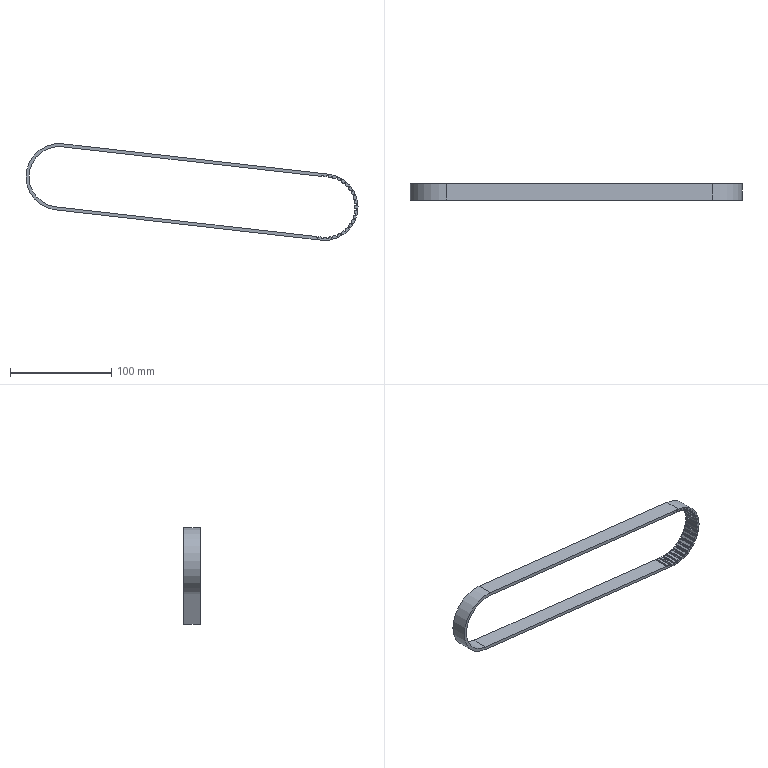Part | STEP file | 冲床-300配套压波_id274_x_t | 1 solid | 196 faces | box 327.52 x 16 x 95.437 mm | volume 33845 mm3 | cylinder 140 | plane 56 | commonest cylinder face diameters 1 x48 3.12 x45 62.52 x24 59.52 x21 65.52 x2